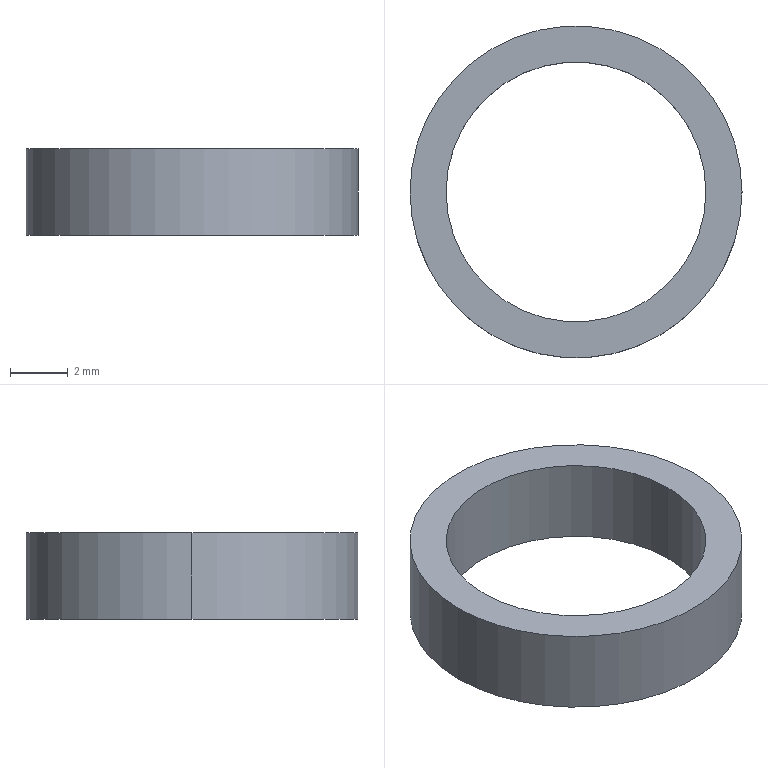Part | NX | features BREP 1 | 1 solid | 6 faces | box 11.5 x 11.5 x 3 mm | volume 120.755 mm3 | cylinder 4 | plane 2 | commonest cylinder face diameters 9 x2 11.5 x2
STEP:
#1=CARTESIAN_POINT('',(4.5,0.,3.));
#2=VERTEX_POINT('',#1);
#3=CARTESIAN_POINT('',(4.5,0.,0.));
#4=VERTEX_POINT('',#3);
#5=CARTESIAN_POINT('',(4.5,0.,3.));
#6=DIRECTION('',(0.,0.,-1.));
#7=VECTOR('',#6,1000.);
#8=LINE('',#5,#7);
#9=EDGE_CURVE('',#2,#4,#8,.T.);
#10=ORIENTED_EDGE('',*,*,#9,.F.);
#11=CARTESIAN_POINT('',(-4.5,0.,3.));
#12=VERTEX_POINT('',#11);
#13=CARTESIAN_POINT('',(0.,0.,3.));
#14=DIRECTION('',(0.,0.,1.));
#15=DIRECTION('',(1.,0.,0.));
#16=AXIS2_PLACEMENT_3D('',#13,#14,#15);
#17=CIRCLE('',#16,4.5);
#18=EDGE_CURVE('',#2,#12,#17,.T.);
#19=ORIENTED_EDGE('',*,*,#18,.T.);
#20=CARTESIAN_POINT('',(-4.5,0.,0.));
#21=VERTEX_POINT('',#20);
#22=CARTESIAN_POINT('',(-4.5,0.,3.));
#23=DIRECTION('',(0.,0.,-1.));
#24=VECTOR('',#23,1000.);
#25=LINE('',#22,#24);
#26=EDGE_CURVE('',#12,#21,#25,.T.);
#27=ORIENTED_EDGE('',*,*,#26,.T.);
#28=CARTESIAN_POINT('',(0.,0.,0.));
#29=DIRECTION('',(0.,0.,1.));
#30=DIRECTION('',(1.,0.,0.));
#31=AXIS2_PLACEMENT_3D('',#28,#29,#30);
#32=CIRCLE('',#31,4.5);
#33=EDGE_CURVE('',#4,#21,#32,.T.);
#34=ORIENTED_EDGE('',*,*,#33,.F.);
#35=EDGE_LOOP('',(#10,#19,#27,#34));
#36=FACE_BOUND('',#35,.T.);
#37=CARTESIAN_POINT('',(0.,0.,3.));
#38=DIRECTION('',(0.,0.,-1.));
#39=DIRECTION('',(-1.,0.,0.));
#40=AXIS2_PLACEMENT_3D('',#37,#38,#39);
#41=CYLINDRICAL_SURFACE('',#40,4.5);
#42=ADVANCED_FACE('',(#36),#41,.F.);
#43=CARTESIAN_POINT('',(5.75,0.,3.));
#44=VERTEX_POINT('',#43);
#45=CARTESIAN_POINT('',(5.75,0.,0.));
#46=VERTEX_POINT('',#45);
#47=CARTESIAN_POINT('',(5.75,0.,3.));
#48=DIRECTION('',(0.,0.,-1.));
#49=VECTOR('',#48,1000.);
#50=LINE('',#47,#49);
#51=EDGE_CURVE('',#44,#46,#50,.T.);
#52=ORIENTED_EDGE('',*,*,#51,.F.);
#53=CARTESIAN_POINT('',(-5.75,0.,3.));
#54=VERTEX_POINT('',#53);
#55=CARTESIAN_POINT('',(0.,0.,3.));
#56=DIRECTION('',(0.,0.,1.));
#57=DIRECTION('',(1.,0.,0.));
#58=AXIS2_PLACEMENT_3D('',#55,#56,#57);
#59=CIRCLE('',#58,5.75);
#60=EDGE_CURVE('',#54,#44,#59,.T.);
#61=ORIENTED_EDGE('',*,*,#60,.F.);
#62=CARTESIAN_POINT('',(-5.75,0.,0.));
#63=VERTEX_POINT('',#62);
#64=CARTESIAN_POINT('',(-5.75,0.,3.));
#65=DIRECTION('',(0.,0.,-1.));
#66=VECTOR('',#65,1000.);
#67=LINE('',#64,#66);
#68=EDGE_CURVE('',#54,#63,#67,.T.);
#69=ORIENTED_EDGE('',*,*,#68,.T.);
#70=CARTESIAN_POINT('',(0.,0.,0.));
#71=DIRECTION('',(0.,0.,1.));
#72=DIRECTION('',(1.,0.,0.));
#73=AXIS2_PLACEMENT_3D('',#70,#71,#72);
#74=CIRCLE('',#73,5.75);
#75=EDGE_CURVE('',#63,#46,#74,.T.);
#76=ORIENTED_EDGE('',*,*,#75,.T.);
#77=EDGE_LOOP('',(#52,#61,#69,#76));
#78=FACE_BOUND('',#77,.T.);
#79=CARTESIAN_POINT('',(0.,0.,3.));
#80=DIRECTION('',(0.,0.,-1.));
#81=DIRECTION('',(-1.,0.,0.));
#82=AXIS2_PLACEMENT_3D('',#79,#80,#81);
#83=CYLINDRICAL_SURFACE('',#82,5.75);
#84=ADVANCED_FACE('',(#78),#83,.T.);
#85=CARTESIAN_POINT('',(0.,0.,0.));
#86=DIRECTION('',(0.,0.,1.));
#87=DIRECTION('',(1.,0.,0.));
#88=AXIS2_PLACEMENT_3D('',#85,#86,#87);
#89=CIRCLE('',#88,4.5);
#90=EDGE_CURVE('',#21,#4,#89,.T.);
#91=ORIENTED_EDGE('',*,*,#90,.T.);
#92=ORIENTED_EDGE('',*,*,#33,.T.);
#93=EDGE_LOOP('',(#91,#92));
#94=FACE_BOUND('',#93,.T.);
#95=ORIENTED_EDGE('',*,*,#75,.F.);
#96=CARTESIAN_POINT('',(0.,0.,0.));
#97=DIRECTION('',(0.,0.,1.));
#98=DIRECTION('',(1.,0.,0.));
#99=AXIS2_PLACEMENT_3D('',#96,#97,#98);
#100=CIRCLE('',#99,5.75);
#101=EDGE_CURVE('',#46,#63,#100,.T.);
#102=ORIENTED_EDGE('',*,*,#101,.F.);
#103=EDGE_LOOP('',(#95,#102));
#104=FACE_BOUND('',#103,.T.);
#105=CARTESIAN_POINT('',(0.,0.,0.));
#106=DIRECTION('',(0.,0.,1.));
#107=DIRECTION('',(1.,0.,0.));
#108=AXIS2_PLACEMENT_3D('',#105,#106,#107);
#109=PLANE('',#108);
#110=ADVANCED_FACE('',(#94,#104),#109,.F.);
#111=CARTESIAN_POINT('',(0.,0.,3.));
#112=DIRECTION('',(0.,0.,1.));
#113=DIRECTION('',(1.,0.,0.));
#114=AXIS2_PLACEMENT_3D('',#111,#112,#113);
#115=CIRCLE('',#114,4.5);
#116=EDGE_CURVE('',#12,#2,#115,.T.);
#117=ORIENTED_EDGE('',*,*,#116,.F.);
#118=ORIENTED_EDGE('',*,*,#18,.F.);
#119=EDGE_LOOP('',(#117,#118));
#120=FACE_BOUND('',#119,.T.);
#121=ORIENTED_EDGE('',*,*,#60,.T.);
#122=CARTESIAN_POINT('',(0.,0.,3.));
#123=DIRECTION('',(0.,0.,1.));
#124=DIRECTION('',(1.,0.,0.));
#125=AXIS2_PLACEMENT_3D('',#122,#123,#124);
#126=CIRCLE('',#125,5.75);
#127=EDGE_CURVE('',#44,#54,#126,.T.);
#128=ORIENTED_EDGE('',*,*,#127,.T.);
#129=EDGE_LOOP('',(#121,#128));
#130=FACE_BOUND('',#129,.T.);
#131=CARTESIAN_POINT('',(0.,0.,3.));
#132=DIRECTION('',(0.,0.,1.));
#133=DIRECTION('',(1.,0.,0.));
#134=AXIS2_PLACEMENT_3D('',#131,#132,#133);
#135=PLANE('',#134);
#136=ADVANCED_FACE('',(#120,#130),#135,.T.);
#137=ORIENTED_EDGE('',*,*,#127,.F.);
#138=ORIENTED_EDGE('',*,*,#51,.T.);
#139=ORIENTED_EDGE('',*,*,#101,.T.);
#140=ORIENTED_EDGE('',*,*,#68,.F.);
#141=EDGE_LOOP('',(#137,#138,#139,#140));
#142=FACE_BOUND('',#141,.T.);
#143=CARTESIAN_POINT('',(0.,0.,3.));
#144=DIRECTION('',(0.,0.,-1.));
#145=DIRECTION('',(-1.,0.,0.));
#146=AXIS2_PLACEMENT_3D('',#143,#144,#145);
#147=CYLINDRICAL_SURFACE('',#146,5.75);
#148=ADVANCED_FACE('',(#142),#147,.T.);
#149=ORIENTED_EDGE('',*,*,#116,.T.);
#150=ORIENTED_EDGE('',*,*,#9,.T.);
#151=ORIENTED_EDGE('',*,*,#90,.F.);
#152=ORIENTED_EDGE('',*,*,#26,.F.);
#153=EDGE_LOOP('',(#149,#150,#151,#152));
#154=FACE_BOUND('',#153,.T.);
#155=CARTESIAN_POINT('',(0.,0.,3.));
#156=DIRECTION('',(0.,0.,-1.));
#157=DIRECTION('',(-1.,0.,0.));
#158=AXIS2_PLACEMENT_3D('',#155,#156,#157);
#159=CYLINDRICAL_SURFACE('',#158,4.5);
#160=ADVANCED_FACE('',(#154),#159,.F.);
#161=CLOSED_SHELL('',(#42,#84,#110,#136,#148,#160));
#162=MANIFOLD_SOLID_BREP('',#161);
#163=(LENGTH_UNIT()NAMED_UNIT(*)SI_UNIT(.MILLI.,.METRE.));
#164=UNCERTAINTY_MEASURE_WITH_UNIT(LENGTH_MEASURE(0.00001),#163,'','');
#165=(NAMED_UNIT(*)PLANE_ANGLE_UNIT()SI_UNIT($,.RADIAN.));
#166=(NAMED_UNIT(*)SI_UNIT($,.STERADIAN.)SOLID_ANGLE_UNIT());
#167=(GEOMETRIC_REPRESENTATION_CONTEXT(3)GLOBAL_UNCERTAINTY_ASSIGNED_CONTEXT((#164))GLOBAL_UNIT_ASSIGNED_CONTEXT((#163,#165,#166))REPRESENTATION_CONTEXT('',''));
#168=ADVANCED_BREP_SHAPE_REPRESENTATION('',(#162),#167);